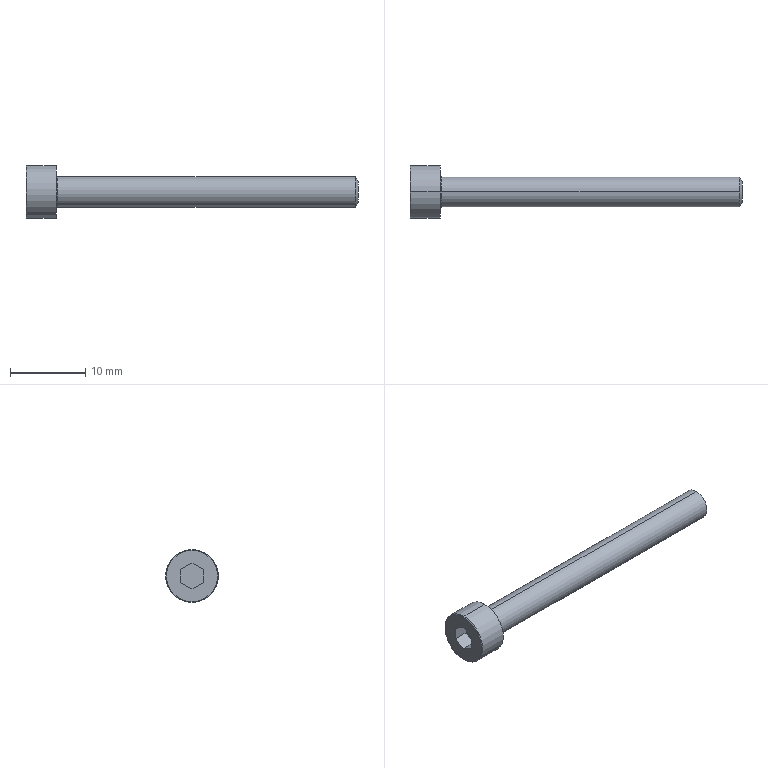Part | SolidWorks | features BlendCut 1, Cut 1, Fillet 1, LPattern 1, RevCut 1, Revolution 1 | 1 solid | 20 faces | box 44 x 7 x 7 mm | volume 640.086 mm3 | plane 10 | torus 4 | cylinder 4 | cone 2 | commonest cylinder face diameters 4 x2 7 x2
STEP:
#1=CARTESIAN_POINT('',(0.,0.,3.4));
#2=VERTEX_POINT('',#1);
#3=CARTESIAN_POINT('',(0.,0.,-3.4));
#4=VERTEX_POINT('',#3);
#5=CARTESIAN_POINT('',(0.,0.,0.));
#6=DIRECTION('',(-1.,0.,0.));
#7=DIRECTION('',(0.,0.,-1.));
#8=AXIS2_PLACEMENT_3D('',#5,#6,#7);
#9=CIRCLE('',#8,3.4);
#10=EDGE_CURVE('',#2,#4,#9,.T.);
#11=ORIENTED_EDGE('',*,*,#10,.F.);
#12=CARTESIAN_POINT('',(0.1,0.,3.5));
#13=VERTEX_POINT('',#12);
#14=CARTESIAN_POINT('',(0.1,0.,3.4));
#15=DIRECTION('',(0.,1.,0.));
#16=DIRECTION('',(0.,0.,1.));
#17=AXIS2_PLACEMENT_3D('',#14,#15,#16);
#18=CIRCLE('',#17,0.1);
#19=EDGE_CURVE('',#2,#13,#18,.T.);
#20=ORIENTED_EDGE('',*,*,#19,.T.);
#21=CARTESIAN_POINT('',(0.1,0.,-3.5));
#22=VERTEX_POINT('',#21);
#23=CARTESIAN_POINT('',(0.1,0.,0.));
#24=DIRECTION('',(1.,0.,0.));
#25=DIRECTION('',(0.,0.,-1.));
#26=AXIS2_PLACEMENT_3D('',#23,#24,#25);
#27=CIRCLE('',#26,3.5);
#28=EDGE_CURVE('',#22,#13,#27,.T.);
#29=ORIENTED_EDGE('',*,*,#28,.F.);
#30=CARTESIAN_POINT('',(0.1,0.,-3.4));
#31=DIRECTION('',(0.,-1.,0.));
#32=DIRECTION('',(0.,0.,-1.));
#33=AXIS2_PLACEMENT_3D('',#30,#31,#32);
#34=CIRCLE('',#33,0.1);
#35=EDGE_CURVE('',#4,#22,#34,.T.);
#36=ORIENTED_EDGE('',*,*,#35,.F.);
#37=EDGE_LOOP('',(#11,#20,#29,#36));
#38=FACE_OUTER_BOUND('',#37,.T.);
#39=CARTESIAN_POINT('',(0.1,0.,0.));
#40=DIRECTION('',(1.,0.,0.));
#41=DIRECTION('',(0.,0.,-1.));
#42=AXIS2_PLACEMENT_3D('',#39,#40,#41);
#43=TOROIDAL_SURFACE('',#42,3.4,0.1);
#44=ADVANCED_FACE('',(#38),#43,.T.);
#45=CARTESIAN_POINT('',(44.,0.,1.394));
#46=VERTEX_POINT('',#45);
#47=CARTESIAN_POINT('',(44.,0.,-1.394));
#48=VERTEX_POINT('',#47);
#49=CARTESIAN_POINT('',(44.,0.,0.));
#50=DIRECTION('',(-1.,0.,0.));
#51=DIRECTION('',(0.,0.,1.));
#52=AXIS2_PLACEMENT_3D('',#49,#50,#51);
#53=CIRCLE('',#52,1.394);
#54=EDGE_CURVE('',#46,#48,#53,.T.);
#55=ORIENTED_EDGE('',*,*,#54,.T.);
#56=CARTESIAN_POINT('',(43.65,0.,-2.));
#57=VERTEX_POINT('',#56);
#58=CARTESIAN_POINT('',(43.65,0.,-2.));
#59=DIRECTION('',(-0.5,0.,-0.866));
#60=VECTOR('',#59,1000.);
#61=LINE('',#58,#60);
#62=EDGE_CURVE('',#48,#57,#61,.T.);
#63=ORIENTED_EDGE('',*,*,#62,.T.);
#64=CARTESIAN_POINT('',(43.65,0.,2.));
#65=VERTEX_POINT('',#64);
#66=CARTESIAN_POINT('',(43.65,0.,0.));
#67=DIRECTION('',(-1.,0.,0.));
#68=DIRECTION('',(0.,0.,1.));
#69=AXIS2_PLACEMENT_3D('',#66,#67,#68);
#70=CIRCLE('',#69,2.);
#71=EDGE_CURVE('',#65,#57,#70,.T.);
#72=ORIENTED_EDGE('',*,*,#71,.F.);
#73=CARTESIAN_POINT('',(43.65,0.,2.));
#74=DIRECTION('',(-0.5,0.,0.866));
#75=VECTOR('',#74,1000.);
#76=LINE('',#73,#75);
#77=EDGE_CURVE('',#46,#65,#76,.T.);
#78=ORIENTED_EDGE('',*,*,#77,.F.);
#79=EDGE_LOOP('',(#55,#63,#72,#78));
#80=FACE_OUTER_BOUND('',#79,.T.);
#81=CARTESIAN_POINT('',(43.65,0.,0.));
#82=DIRECTION('',(-1.,0.,0.));
#83=DIRECTION('',(0.,0.,1.));
#84=AXIS2_PLACEMENT_3D('',#81,#82,#83);
#85=CONICAL_SURFACE('',#84,2.,1.047);
#86=ADVANCED_FACE('',(#80),#85,.T.);
#87=CARTESIAN_POINT('',(4.,0.,-2.2));
#88=VERTEX_POINT('',#87);
#89=CARTESIAN_POINT('',(4.,0.,2.2));
#90=VERTEX_POINT('',#89);
#91=CARTESIAN_POINT('',(4.,0.,0.));
#92=DIRECTION('',(-1.,0.,0.));
#93=DIRECTION('',(0.,0.,1.));
#94=AXIS2_PLACEMENT_3D('',#91,#92,#93);
#95=CIRCLE('',#94,2.2);
#96=EDGE_CURVE('',#88,#90,#95,.T.);
#97=ORIENTED_EDGE('',*,*,#96,.F.);
#98=CARTESIAN_POINT('',(4.2,0.,-2.));
#99=VERTEX_POINT('',#98);
#100=CARTESIAN_POINT('',(4.2,0.,-2.2));
#101=DIRECTION('',(0.,1.,0.));
#102=DIRECTION('',(0.,0.,1.));
#103=AXIS2_PLACEMENT_3D('',#100,#101,#102);
#104=CIRCLE('',#103,0.2);
#105=EDGE_CURVE('',#88,#99,#104,.T.);
#106=ORIENTED_EDGE('',*,*,#105,.T.);
#107=CARTESIAN_POINT('',(4.2,0.,2.));
#108=VERTEX_POINT('',#107);
#109=CARTESIAN_POINT('',(4.2,0.,0.));
#110=DIRECTION('',(-1.,0.,0.));
#111=DIRECTION('',(0.,0.,1.));
#112=AXIS2_PLACEMENT_3D('',#109,#110,#111);
#113=CIRCLE('',#112,2.);
#114=EDGE_CURVE('',#99,#108,#113,.T.);
#115=ORIENTED_EDGE('',*,*,#114,.T.);
#116=CARTESIAN_POINT('',(4.2,0.,2.2));
#117=DIRECTION('',(0.,-1.,0.));
#118=DIRECTION('',(0.,0.,-1.));
#119=AXIS2_PLACEMENT_3D('',#116,#117,#118);
#120=CIRCLE('',#119,0.2);
#121=EDGE_CURVE('',#90,#108,#120,.T.);
#122=ORIENTED_EDGE('',*,*,#121,.F.);
#123=EDGE_LOOP('',(#97,#106,#115,#122));
#124=FACE_OUTER_BOUND('',#123,.T.);
#125=CARTESIAN_POINT('',(4.2,0.,0.));
#126=DIRECTION('',(-1.,0.,0.));
#127=DIRECTION('',(0.,0.,1.));
#128=AXIS2_PLACEMENT_3D('',#125,#126,#127);
#129=TOROIDAL_SURFACE('',#128,2.2,0.2);
#130=ADVANCED_FACE('',(#124),#129,.F.);
#131=CARTESIAN_POINT('',(4.,0.,3.5));
#132=VERTEX_POINT('',#131);
#133=CARTESIAN_POINT('',(4.,0.,-3.5));
#134=VERTEX_POINT('',#133);
#135=CARTESIAN_POINT('',(4.,0.,0.));
#136=DIRECTION('',(-1.,0.,0.));
#137=DIRECTION('',(0.,0.,1.));
#138=AXIS2_PLACEMENT_3D('',#135,#136,#137);
#139=CIRCLE('',#138,3.5);
#140=EDGE_CURVE('',#132,#134,#139,.T.);
#141=ORIENTED_EDGE('',*,*,#140,.T.);
#142=CARTESIAN_POINT('',(0.,0.,-3.5));
#143=DIRECTION('',(-1.,0.,0.));
#144=VECTOR('',#143,1000.);
#145=LINE('',#142,#144);
#146=EDGE_CURVE('',#134,#22,#145,.T.);
#147=ORIENTED_EDGE('',*,*,#146,.T.);
#148=ORIENTED_EDGE('',*,*,#28,.T.);
#149=CARTESIAN_POINT('',(0.,0.,3.5));
#150=DIRECTION('',(-1.,0.,0.));
#151=VECTOR('',#150,1000.);
#152=LINE('',#149,#151);
#153=EDGE_CURVE('',#132,#13,#152,.T.);
#154=ORIENTED_EDGE('',*,*,#153,.F.);
#155=EDGE_LOOP('',(#141,#147,#148,#154));
#156=FACE_OUTER_BOUND('',#155,.T.);
#157=CARTESIAN_POINT('',(0.,0.,0.));
#158=DIRECTION('',(-1.,0.,0.));
#159=DIRECTION('',(0.,0.,1.));
#160=AXIS2_PLACEMENT_3D('',#157,#158,#159);
#161=CYLINDRICAL_SURFACE('',#160,3.5);
#162=ADVANCED_FACE('',(#156),#161,.T.);
#163=ORIENTED_EDGE('',*,*,#71,.T.);
#164=CARTESIAN_POINT('',(0.,0.,-2.));
#165=DIRECTION('',(-1.,0.,0.));
#166=VECTOR('',#165,1000.);
#167=LINE('',#164,#166);
#168=EDGE_CURVE('',#57,#99,#167,.T.);
#169=ORIENTED_EDGE('',*,*,#168,.T.);
#170=CARTESIAN_POINT('',(4.2,0.,0.));
#171=DIRECTION('',(-1.,0.,0.));
#172=DIRECTION('',(0.,0.,1.));
#173=AXIS2_PLACEMENT_3D('',#170,#171,#172);
#174=CIRCLE('',#173,2.);
#175=EDGE_CURVE('',#108,#99,#174,.T.);
#176=ORIENTED_EDGE('',*,*,#175,.F.);
#177=CARTESIAN_POINT('',(0.,0.,2.));
#178=DIRECTION('',(-1.,0.,0.));
#179=VECTOR('',#178,1000.);
#180=LINE('',#177,#179);
#181=EDGE_CURVE('',#65,#108,#180,.T.);
#182=ORIENTED_EDGE('',*,*,#181,.F.);
#183=EDGE_LOOP('',(#163,#169,#176,#182));
#184=FACE_OUTER_BOUND('',#183,.T.);
#185=CARTESIAN_POINT('',(0.,0.,0.));
#186=DIRECTION('',(-1.,0.,0.));
#187=DIRECTION('',(0.,0.,1.));
#188=AXIS2_PLACEMENT_3D('',#185,#186,#187);
#189=CYLINDRICAL_SURFACE('',#188,2.);
#190=ADVANCED_FACE('',(#184),#189,.T.);
#191=ORIENTED_EDGE('',*,*,#168,.F.);
#192=CARTESIAN_POINT('',(43.65,0.,0.));
#193=DIRECTION('',(-1.,0.,0.));
#194=DIRECTION('',(0.,0.,1.));
#195=AXIS2_PLACEMENT_3D('',#192,#193,#194);
#196=CIRCLE('',#195,2.);
#197=EDGE_CURVE('',#57,#65,#196,.T.);
#198=ORIENTED_EDGE('',*,*,#197,.T.);
#199=ORIENTED_EDGE('',*,*,#181,.T.);
#200=ORIENTED_EDGE('',*,*,#114,.F.);
#201=EDGE_LOOP('',(#191,#198,#199,#200));
#202=FACE_OUTER_BOUND('',#201,.T.);
#203=CARTESIAN_POINT('',(0.,0.,0.));
#204=DIRECTION('',(-1.,0.,0.));
#205=DIRECTION('',(0.,0.,1.));
#206=AXIS2_PLACEMENT_3D('',#203,#204,#205);
#207=CYLINDRICAL_SURFACE('',#206,2.);
#208=ADVANCED_FACE('',(#202),#207,.T.);
#209=CARTESIAN_POINT('',(0.,0.,0.));
#210=DIRECTION('',(-1.,0.,0.));
#211=DIRECTION('',(0.,0.,-1.));
#212=AXIS2_PLACEMENT_3D('',#209,#210,#211);
#213=CIRCLE('',#212,3.4);
#214=EDGE_CURVE('',#4,#2,#213,.T.);
#215=ORIENTED_EDGE('',*,*,#214,.T.);
#216=ORIENTED_EDGE('',*,*,#10,.T.);
#217=EDGE_LOOP('',(#215,#216));
#218=FACE_OUTER_BOUND('',#217,.T.);
#219=CARTESIAN_POINT('',(0.,0.,1.72));
#220=VERTEX_POINT('',#219);
#221=CARTESIAN_POINT('',(0.,1.49,0.86));
#222=VERTEX_POINT('',#221);
#223=CARTESIAN_POINT('',(0.,0.,1.72));
#224=DIRECTION('',(0.,0.866,-0.5));
#225=VECTOR('',#224,1000.);
#226=LINE('',#223,#225);
#227=EDGE_CURVE('',#220,#222,#226,.T.);
#228=ORIENTED_EDGE('',*,*,#227,.F.);
#229=CARTESIAN_POINT('',(0.,-1.49,0.86));
#230=VERTEX_POINT('',#229);
#231=CARTESIAN_POINT('',(0.,-1.49,0.86));
#232=DIRECTION('',(0.,0.866,0.5));
#233=VECTOR('',#232,1000.);
#234=LINE('',#231,#233);
#235=EDGE_CURVE('',#230,#220,#234,.T.);
#236=ORIENTED_EDGE('',*,*,#235,.F.);
#237=CARTESIAN_POINT('',(0.,-1.49,-0.86));
#238=VERTEX_POINT('',#237);
#239=CARTESIAN_POINT('',(0.,-1.49,-0.86));
#240=DIRECTION('',(0.,0.,1.));
#241=VECTOR('',#240,1000.);
#242=LINE('',#239,#241);
#243=EDGE_CURVE('',#238,#230,#242,.T.);
#244=ORIENTED_EDGE('',*,*,#243,.F.);
#245=CARTESIAN_POINT('',(0.,0.,-1.72));
#246=VERTEX_POINT('',#245);
#247=CARTESIAN_POINT('',(0.,0.,-1.72));
#248=DIRECTION('',(0.,-0.866,0.5));
#249=VECTOR('',#248,1000.);
#250=LINE('',#247,#249);
#251=EDGE_CURVE('',#246,#238,#250,.T.);
#252=ORIENTED_EDGE('',*,*,#251,.F.);
#253=CARTESIAN_POINT('',(0.,1.49,-0.86));
#254=VERTEX_POINT('',#253);
#255=CARTESIAN_POINT('',(0.,1.49,-0.86));
#256=DIRECTION('',(0.,-0.866,-0.5));
#257=VECTOR('',#256,1000.);
#258=LINE('',#255,#257);
#259=EDGE_CURVE('',#254,#246,#258,.T.);
#260=ORIENTED_EDGE('',*,*,#259,.F.);
#261=CARTESIAN_POINT('',(0.,1.49,0.86));
#262=DIRECTION('',(0.,0.,-1.));
#263=VECTOR('',#262,1000.);
#264=LINE('',#261,#263);
#265=EDGE_CURVE('',#222,#254,#264,.T.);
#266=ORIENTED_EDGE('',*,*,#265,.F.);
#267=EDGE_LOOP('',(#228,#236,#244,#252,#260,#266));
#268=FACE_BOUND('',#267,.T.);
#269=CARTESIAN_POINT('',(0.,0.,0.));
#270=DIRECTION('',(1.,0.,0.));
#271=DIRECTION('',(0.,0.,-1.));
#272=AXIS2_PLACEMENT_3D('',#269,#270,#271);
#273=PLANE('',#272);
#274=ADVANCED_FACE('',(#218,#268),#273,.F.);
#275=ORIENTED_EDGE('',*,*,#146,.F.);
#276=CARTESIAN_POINT('',(4.,0.,0.));
#277=DIRECTION('',(-1.,0.,0.));
#278=DIRECTION('',(0.,0.,1.));
#279=AXIS2_PLACEMENT_3D('',#276,#277,#278);
#280=CIRCLE('',#279,3.5);
#281=EDGE_CURVE('',#134,#132,#280,.T.);
#282=ORIENTED_EDGE('',*,*,#281,.T.);
#283=ORIENTED_EDGE('',*,*,#153,.T.);
#284=CARTESIAN_POINT('',(0.1,0.,0.));
#285=DIRECTION('',(1.,0.,0.));
#286=DIRECTION('',(0.,0.,-1.));
#287=AXIS2_PLACEMENT_3D('',#284,#285,#286);
#288=CIRCLE('',#287,3.5);
#289=EDGE_CURVE('',#13,#22,#288,.T.);
#290=ORIENTED_EDGE('',*,*,#289,.T.);
#291=EDGE_LOOP('',(#275,#282,#283,#290));
#292=FACE_OUTER_BOUND('',#291,.T.);
#293=CARTESIAN_POINT('',(0.,0.,0.));
#294=DIRECTION('',(-1.,0.,0.));
#295=DIRECTION('',(0.,0.,1.));
#296=AXIS2_PLACEMENT_3D('',#293,#294,#295);
#297=CYLINDRICAL_SURFACE('',#296,3.5);
#298=ADVANCED_FACE('',(#292),#297,.T.);
#299=ORIENTED_EDGE('',*,*,#140,.F.);
#300=ORIENTED_EDGE('',*,*,#281,.F.);
#301=EDGE_LOOP('',(#299,#300));
#302=FACE_OUTER_BOUND('',#301,.T.);
#303=CARTESIAN_POINT('',(4.,0.,0.));
#304=DIRECTION('',(-1.,0.,0.));
#305=DIRECTION('',(0.,0.,1.));
#306=AXIS2_PLACEMENT_3D('',#303,#304,#305);
#307=CIRCLE('',#306,2.2);
#308=EDGE_CURVE('',#90,#88,#307,.T.);
#309=ORIENTED_EDGE('',*,*,#308,.T.);
#310=ORIENTED_EDGE('',*,*,#96,.T.);
#311=EDGE_LOOP('',(#309,#310));
#312=FACE_BOUND('',#311,.T.);
#313=CARTESIAN_POINT('',(4.,3.5,0.));
#314=DIRECTION('',(-1.,0.,0.));
#315=DIRECTION('',(0.,0.,1.));
#316=AXIS2_PLACEMENT_3D('',#313,#314,#315);
#317=PLANE('',#316);
#318=ADVANCED_FACE('',(#302,#312),#317,.F.);
#319=ORIENTED_EDGE('',*,*,#105,.F.);
#320=ORIENTED_EDGE('',*,*,#308,.F.);
#321=ORIENTED_EDGE('',*,*,#121,.T.);
#322=ORIENTED_EDGE('',*,*,#175,.T.);
#323=EDGE_LOOP('',(#319,#320,#321,#322));
#324=FACE_OUTER_BOUND('',#323,.T.);
#325=CARTESIAN_POINT('',(4.2,0.,0.));
#326=DIRECTION('',(-1.,0.,0.));
#327=DIRECTION('',(0.,0.,1.));
#328=AXIS2_PLACEMENT_3D('',#325,#326,#327);
#329=TOROIDAL_SURFACE('',#328,2.2,0.2);
#330=ADVANCED_FACE('',(#324),#329,.F.);
#331=ORIENTED_EDGE('',*,*,#235,.T.);
#332=CARTESIAN_POINT('',(2.,0.,1.72));
#333=VERTEX_POINT('',#332);
#334=CARTESIAN_POINT('',(2.,0.,1.72));
#335=DIRECTION('',(-1.,0.,0.));
#336=VECTOR('',#335,1000.);
#337=LINE('',#334,#336);
#338=EDGE_CURVE('',#333,#220,#337,.T.);
#339=ORIENTED_EDGE('',*,*,#338,.F.);
#340=CARTESIAN_POINT('',(2.,-1.49,0.86));
#341=VERTEX_POINT('',#340);
#342=CARTESIAN_POINT('',(2.,-1.49,0.86));
#343=DIRECTION('',(0.,0.866,0.5));
#344=VECTOR('',#343,1000.);
#345=LINE('',#342,#344);
#346=EDGE_CURVE('',#341,#333,#345,.T.);
#347=ORIENTED_EDGE('',*,*,#346,.F.);
#348=CARTESIAN_POINT('',(2.,-1.49,0.86));
#349=DIRECTION('',(-1.,0.,0.));
#350=VECTOR('',#349,1000.);
#351=LINE('',#348,#350);
#352=EDGE_CURVE('',#341,#230,#351,.T.);
#353=ORIENTED_EDGE('',*,*,#352,.T.);
#354=EDGE_LOOP('',(#331,#339,#347,#353));
#355=FACE_OUTER_BOUND('',#354,.T.);
#356=CARTESIAN_POINT('',(2.,-1.49,0.86));
#357=DIRECTION('',(0.,-0.5,0.866));
#358=DIRECTION('',(0.,-0.866,-0.5));
#359=AXIS2_PLACEMENT_3D('',#356,#357,#358);
#360=PLANE('',#359);
#361=ADVANCED_FACE('',(#355),#360,.F.);
#362=ORIENTED_EDGE('',*,*,#243,.T.);
#363=ORIENTED_EDGE('',*,*,#352,.F.);
#364=CARTESIAN_POINT('',(2.,-1.49,-0.86));
#365=VERTEX_POINT('',#364);
#366=CARTESIAN_POINT('',(2.,-1.49,-0.86));
#367=DIRECTION('',(0.,0.,1.));
#368=VECTOR('',#367,1000.);
#369=LINE('',#366,#368);
#370=EDGE_CURVE('',#365,#341,#369,.T.);
#371=ORIENTED_EDGE('',*,*,#370,.F.);
#372=CARTESIAN_POINT('',(2.,-1.49,-0.86));
#373=DIRECTION('',(-1.,0.,0.));
#374=VECTOR('',#373,1000.);
#375=LINE('',#372,#374);
#376=EDGE_CURVE('',#365,#238,#375,.T.);
#377=ORIENTED_EDGE('',*,*,#376,.T.);
#378=EDGE_LOOP('',(#362,#363,#371,#377));
#379=FACE_OUTER_BOUND('',#378,.T.);
#380=CARTESIAN_POINT('',(2.,-1.49,-0.86));
#381=DIRECTION('',(0.,-1.,0.));
#382=DIRECTION('',(0.,0.,-1.));
#383=AXIS2_PLACEMENT_3D('',#380,#381,#382);
#384=PLANE('',#383);
#385=ADVANCED_FACE('',(#379),#384,.F.);
#386=ORIENTED_EDGE('',*,*,#251,.T.);
#387=ORIENTED_EDGE('',*,*,#376,.F.);
#388=CARTESIAN_POINT('',(2.,0.,-1.72));
#389=VERTEX_POINT('',#388);
#390=CARTESIAN_POINT('',(2.,0.,-1.72));
#391=DIRECTION('',(0.,-0.866,0.5));
#392=VECTOR('',#391,1000.);
#393=LINE('',#390,#392);
#394=EDGE_CURVE('',#389,#365,#393,.T.);
#395=ORIENTED_EDGE('',*,*,#394,.F.);
#396=CARTESIAN_POINT('',(2.,0.,-1.72));
#397=DIRECTION('',(-1.,0.,0.));
#398=VECTOR('',#397,1000.);
#399=LINE('',#396,#398);
#400=EDGE_CURVE('',#389,#246,#399,.T.);
#401=ORIENTED_EDGE('',*,*,#400,.T.);
#402=EDGE_LOOP('',(#386,#387,#395,#401));
#403=FACE_OUTER_BOUND('',#402,.T.);
#404=CARTESIAN_POINT('',(2.,0.,-1.72));
#405=DIRECTION('',(0.,-0.5,-0.866));
#406=DIRECTION('',(0.,0.866,-0.5));
#407=AXIS2_PLACEMENT_3D('',#404,#405,#406);
#408=PLANE('',#407);
#409=ADVANCED_FACE('',(#403),#408,.F.);
#410=ORIENTED_EDGE('',*,*,#259,.T.);
#411=ORIENTED_EDGE('',*,*,#400,.F.);
#412=CARTESIAN_POINT('',(2.,1.49,-0.86));
#413=VERTEX_POINT('',#412);
#414=CARTESIAN_POINT('',(2.,1.49,-0.86));
#415=DIRECTION('',(0.,-0.866,-0.5));
#416=VECTOR('',#415,1000.);
#417=LINE('',#414,#416);
#418=EDGE_CURVE('',#413,#389,#417,.T.);
#419=ORIENTED_EDGE('',*,*,#418,.F.);
#420=CARTESIAN_POINT('',(2.,1.49,-0.86));
#421=DIRECTION('',(-1.,0.,0.));
#422=VECTOR('',#421,1000.);
#423=LINE('',#420,#422);
#424=EDGE_CURVE('',#413,#254,#423,.T.);
#425=ORIENTED_EDGE('',*,*,#424,.T.);
#426=EDGE_LOOP('',(#410,#411,#419,#425));
#427=FACE_OUTER_BOUND('',#426,.T.);
#428=CARTESIAN_POINT('',(2.,1.49,-0.86));
#429=DIRECTION('',(0.,0.5,-0.866));
#430=DIRECTION('',(0.,0.866,0.5));
#431=AXIS2_PLACEMENT_3D('',#428,#429,#430);
#432=PLANE('',#431);
#433=ADVANCED_FACE('',(#427),#432,.F.);
#434=ORIENTED_EDGE('',*,*,#265,.T.);
#435=ORIENTED_EDGE('',*,*,#424,.F.);
#436=CARTESIAN_POINT('',(2.,1.49,0.86));
#437=VERTEX_POINT('',#436);
#438=CARTESIAN_POINT('',(2.,1.49,0.86));
#439=DIRECTION('',(0.,0.,-1.));
#440=VECTOR('',#439,1000.);
#441=LINE('',#438,#440);
#442=EDGE_CURVE('',#437,#413,#441,.T.);
#443=ORIENTED_EDGE('',*,*,#442,.F.);
#444=CARTESIAN_POINT('',(2.,1.49,0.86));
#445=DIRECTION('',(-1.,0.,0.));
#446=VECTOR('',#445,1000.);
#447=LINE('',#444,#446);
#448=EDGE_CURVE('',#437,#222,#447,.T.);
#449=ORIENTED_EDGE('',*,*,#448,.T.);
#450=EDGE_LOOP('',(#434,#435,#443,#449));
#451=FACE_OUTER_BOUND('',#450,.T.);
#452=CARTESIAN_POINT('',(2.,1.49,0.86));
#453=DIRECTION('',(0.,1.,0.));
#454=DIRECTION('',(0.,0.,1.));
#455=AXIS2_PLACEMENT_3D('',#452,#453,#454);
#456=PLANE('',#455);
#457=ADVANCED_FACE('',(#451),#456,.F.);
#458=ORIENTED_EDGE('',*,*,#227,.T.);
#459=ORIENTED_EDGE('',*,*,#448,.F.);
#460=CARTESIAN_POINT('',(2.,0.,1.72));
#461=DIRECTION('',(0.,0.866,-0.5));
#462=VECTOR('',#461,1000.);
#463=LINE('',#460,#462);
#464=EDGE_CURVE('',#333,#437,#463,.T.);
#465=ORIENTED_EDGE('',*,*,#464,.F.);
#466=ORIENTED_EDGE('',*,*,#338,.T.);
#467=EDGE_LOOP('',(#458,#459,#465,#466));
#468=FACE_OUTER_BOUND('',#467,.T.);
#469=CARTESIAN_POINT('',(2.,0.,1.72));
#470=DIRECTION('',(0.,0.5,0.866));
#471=DIRECTION('',(0.,-0.866,0.5));
#472=AXIS2_PLACEMENT_3D('',#469,#470,#471);
#473=PLANE('',#472);
#474=ADVANCED_FACE('',(#468),#473,.F.);
#475=ORIENTED_EDGE('',*,*,#346,.T.);
#476=ORIENTED_EDGE('',*,*,#464,.T.);
#477=ORIENTED_EDGE('',*,*,#442,.T.);
#478=ORIENTED_EDGE('',*,*,#418,.T.);
#479=ORIENTED_EDGE('',*,*,#394,.T.);
#480=ORIENTED_EDGE('',*,*,#370,.T.);
#481=EDGE_LOOP('',(#475,#476,#477,#478,#479,#480));
#482=FACE_OUTER_BOUND('',#481,.T.);
#483=CARTESIAN_POINT('',(2.,1.49,2.58));
#484=DIRECTION('',(-1.,0.,0.));
#485=DIRECTION('',(0.,0.,1.));
#486=AXIS2_PLACEMENT_3D('',#483,#484,#485);
#487=PLANE('',#486);
#488=ADVANCED_FACE('',(#482),#487,.T.);
#489=ORIENTED_EDGE('',*,*,#62,.F.);
#490=CARTESIAN_POINT('',(44.,0.,0.));
#491=DIRECTION('',(-1.,0.,0.));
#492=DIRECTION('',(0.,0.,1.));
#493=AXIS2_PLACEMENT_3D('',#490,#491,#492);
#494=CIRCLE('',#493,1.394);
#495=EDGE_CURVE('',#48,#46,#494,.T.);
#496=ORIENTED_EDGE('',*,*,#495,.T.);
#497=ORIENTED_EDGE('',*,*,#77,.T.);
#498=ORIENTED_EDGE('',*,*,#197,.F.);
#499=EDGE_LOOP('',(#489,#496,#497,#498));
#500=FACE_OUTER_BOUND('',#499,.T.);
#501=CARTESIAN_POINT('',(43.65,0.,0.));
#502=DIRECTION('',(-1.,0.,0.));
#503=DIRECTION('',(0.,0.,1.));
#504=AXIS2_PLACEMENT_3D('',#501,#502,#503);
#505=CONICAL_SURFACE('',#504,2.,1.047);
#506=ADVANCED_FACE('',(#500),#505,.T.);
#507=ORIENTED_EDGE('',*,*,#54,.F.);
#508=ORIENTED_EDGE('',*,*,#495,.F.);
#509=EDGE_LOOP('',(#507,#508));
#510=FACE_OUTER_BOUND('',#509,.T.);
#511=CARTESIAN_POINT('',(44.,2.,0.));
#512=DIRECTION('',(-1.,0.,0.));
#513=DIRECTION('',(0.,0.,1.));
#514=AXIS2_PLACEMENT_3D('',#511,#512,#513);
#515=PLANE('',#514);
#516=ADVANCED_FACE('',(#510),#515,.F.);
#517=ORIENTED_EDGE('',*,*,#19,.F.);
#518=ORIENTED_EDGE('',*,*,#214,.F.);
#519=ORIENTED_EDGE('',*,*,#35,.T.);
#520=ORIENTED_EDGE('',*,*,#289,.F.);
#521=EDGE_LOOP('',(#517,#518,#519,#520));
#522=FACE_OUTER_BOUND('',#521,.T.);
#523=CARTESIAN_POINT('',(0.1,0.,0.));
#524=DIRECTION('',(1.,0.,0.));
#525=DIRECTION('',(0.,0.,-1.));
#526=AXIS2_PLACEMENT_3D('',#523,#524,#525);
#527=TOROIDAL_SURFACE('',#526,3.4,0.1);
#528=ADVANCED_FACE('',(#522),#527,.T.);
#529=CLOSED_SHELL('',(#44,#86,#130,#162,#190,#208,#274,#298,#318,#330,#361,#385,#409,#433,#457,#474,#488,#506,#516,#528));
#530=MANIFOLD_SOLID_BREP('',#529);
#531=CARTESIAN_POINT('',(0.,0.,0.));
#532=DIRECTION('',(0.,0.,1.));
#533=DIRECTION('',(1.,0.,0.));
#534=AXIS2_PLACEMENT_3D('',#531,#532,#533);
#535=(LENGTH_UNIT()NAMED_UNIT(*)SI_UNIT(.MILLI.,.METRE.));
#536=UNCERTAINTY_MEASURE_WITH_UNIT(LENGTH_MEASURE(0.00001),#535,'','');
#537=(NAMED_UNIT(*)PLANE_ANGLE_UNIT()SI_UNIT($,.RADIAN.));
#538=(NAMED_UNIT(*)SI_UNIT($,.STERADIAN.)SOLID_ANGLE_UNIT());
#539=(GEOMETRIC_REPRESENTATION_CONTEXT(3)GLOBAL_UNCERTAINTY_ASSIGNED_CONTEXT((#536))GLOBAL_UNIT_ASSIGNED_CONTEXT((#535,#537,#538))REPRESENTATION_CONTEXT('',''));
#540=ADVANCED_BREP_SHAPE_REPRESENTATION('',(#530,#534),#539);